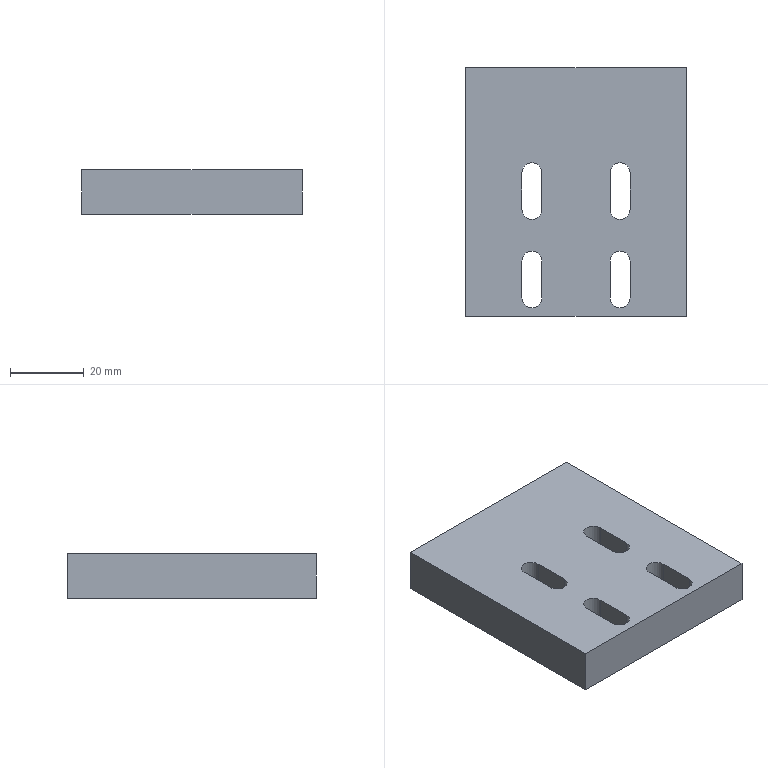Part | SolidWorks | features Cut 1, Extrusion 1, HoleWzd 1 | 1 solid | 30 faces | box 60 x 67.5 x 12 mm | volume 44553 mm3 | plane 14 | cylinder 12 | cone 4 | commonest cylinder face diameters 5.4 x8 4.2 x4
STEP:
#1=CARTESIAN_POINT('',(-15.,21.35,-2.1));
#2=VERTEX_POINT('',#1);
#3=CARTESIAN_POINT('',(-15.,21.35,2.1));
#4=VERTEX_POINT('',#3);
#5=CARTESIAN_POINT('',(-15.,21.35,0.));
#6=DIRECTION('',(0.,1.,0.));
#7=DIRECTION('',(0.,0.,1.));
#8=AXIS2_PLACEMENT_3D('',#5,#6,#7);
#9=CIRCLE('',#8,2.1);
#10=EDGE_CURVE('',#2,#4,#9,.T.);
#11=ORIENTED_EDGE('',*,*,#10,.F.);
#12=CARTESIAN_POINT('',(-15.,33.75,-2.1));
#13=VERTEX_POINT('',#12);
#14=CARTESIAN_POINT('',(-15.,33.75,-2.1));
#15=DIRECTION('',(0.,1.,0.));
#16=VECTOR('',#15,1000.);
#17=LINE('',#14,#16);
#18=EDGE_CURVE('',#2,#13,#17,.T.);
#19=ORIENTED_EDGE('',*,*,#18,.T.);
#20=CARTESIAN_POINT('',(-15.,33.75,2.1));
#21=VERTEX_POINT('',#20);
#22=CARTESIAN_POINT('',(-15.,33.75,0.));
#23=DIRECTION('',(0.,1.,0.));
#24=DIRECTION('',(0.,0.,1.));
#25=AXIS2_PLACEMENT_3D('',#22,#23,#24);
#26=CIRCLE('',#25,2.1);
#27=EDGE_CURVE('',#13,#21,#26,.T.);
#28=ORIENTED_EDGE('',*,*,#27,.T.);
#29=CARTESIAN_POINT('',(-15.,33.75,2.1));
#30=DIRECTION('',(0.,1.,0.));
#31=VECTOR('',#30,1000.);
#32=LINE('',#29,#31);
#33=EDGE_CURVE('',#4,#21,#32,.T.);
#34=ORIENTED_EDGE('',*,*,#33,.F.);
#35=EDGE_LOOP('',(#11,#19,#28,#34));
#36=FACE_OUTER_BOUND('',#35,.T.);
#37=CARTESIAN_POINT('',(-15.,33.75,0.));
#38=DIRECTION('',(0.,1.,0.));
#39=DIRECTION('',(0.,0.,1.));
#40=AXIS2_PLACEMENT_3D('',#37,#38,#39);
#41=CYLINDRICAL_SURFACE('',#40,2.1);
#42=ADVANCED_FACE('',(#36),#41,.F.);
#43=CARTESIAN_POINT('',(-15.,20.088,0.));
#44=VERTEX_POINT('',#43);
#45=CARTESIAN_POINT('',(-15.,21.35,2.1));
#46=DIRECTION('',(0.,0.515,0.8572));
#47=VECTOR('',#46,1000.);
#48=LINE('',#45,#47);
#49=EDGE_CURVE('',#44,#4,#48,.T.);
#50=ORIENTED_EDGE('',*,*,#49,.F.);
#51=CARTESIAN_POINT('',(-15.,21.35,-2.1));
#52=DIRECTION('',(0.,0.515,-0.8572));
#53=VECTOR('',#52,1000.);
#54=LINE('',#51,#53);
#55=EDGE_CURVE('',#44,#2,#54,.T.);
#56=ORIENTED_EDGE('',*,*,#55,.T.);
#57=ORIENTED_EDGE('',*,*,#10,.T.);
#58=EDGE_LOOP('',(#50,#56,#57));
#59=FACE_OUTER_BOUND('',#58,.T.);
#60=CARTESIAN_POINT('',(-15.,21.35,0.));
#61=DIRECTION('',(0.,1.,0.));
#62=DIRECTION('',(0.,0.,1.));
#63=AXIS2_PLACEMENT_3D('',#60,#61,#62);
#64=CONICAL_SURFACE('',#63,2.1,1.03);
#65=ADVANCED_FACE('',(#59),#64,.F.);
#66=CARTESIAN_POINT('',(15.,21.35,-2.1));
#67=VERTEX_POINT('',#66);
#68=CARTESIAN_POINT('',(15.,21.35,2.1));
#69=VERTEX_POINT('',#68);
#70=CARTESIAN_POINT('',(15.,21.35,0.));
#71=DIRECTION('',(0.,1.,0.));
#72=DIRECTION('',(0.,0.,1.));
#73=AXIS2_PLACEMENT_3D('',#70,#71,#72);
#74=CIRCLE('',#73,2.1);
#75=EDGE_CURVE('',#67,#69,#74,.T.);
#76=ORIENTED_EDGE('',*,*,#75,.F.);
#77=CARTESIAN_POINT('',(15.,33.75,-2.1));
#78=VERTEX_POINT('',#77);
#79=CARTESIAN_POINT('',(15.,33.75,-2.1));
#80=DIRECTION('',(0.,1.,0.));
#81=VECTOR('',#80,1000.);
#82=LINE('',#79,#81);
#83=EDGE_CURVE('',#67,#78,#82,.T.);
#84=ORIENTED_EDGE('',*,*,#83,.T.);
#85=CARTESIAN_POINT('',(15.,33.75,2.1));
#86=VERTEX_POINT('',#85);
#87=CARTESIAN_POINT('',(15.,33.75,0.));
#88=DIRECTION('',(0.,1.,0.));
#89=DIRECTION('',(0.,0.,1.));
#90=AXIS2_PLACEMENT_3D('',#87,#88,#89);
#91=CIRCLE('',#90,2.1);
#92=EDGE_CURVE('',#78,#86,#91,.T.);
#93=ORIENTED_EDGE('',*,*,#92,.T.);
#94=CARTESIAN_POINT('',(15.,33.75,2.1));
#95=DIRECTION('',(0.,1.,0.));
#96=VECTOR('',#95,1000.);
#97=LINE('',#94,#96);
#98=EDGE_CURVE('',#69,#86,#97,.T.);
#99=ORIENTED_EDGE('',*,*,#98,.F.);
#100=EDGE_LOOP('',(#76,#84,#93,#99));
#101=FACE_OUTER_BOUND('',#100,.T.);
#102=CARTESIAN_POINT('',(15.,33.75,0.));
#103=DIRECTION('',(0.,1.,0.));
#104=DIRECTION('',(0.,0.,1.));
#105=AXIS2_PLACEMENT_3D('',#102,#103,#104);
#106=CYLINDRICAL_SURFACE('',#105,2.1);
#107=ADVANCED_FACE('',(#101),#106,.F.);
#108=CARTESIAN_POINT('',(15.,20.088,0.));
#109=VERTEX_POINT('',#108);
#110=CARTESIAN_POINT('',(15.,21.35,2.1));
#111=DIRECTION('',(0.,0.515,0.8572));
#112=VECTOR('',#111,1000.);
#113=LINE('',#110,#112);
#114=EDGE_CURVE('',#109,#69,#113,.T.);
#115=ORIENTED_EDGE('',*,*,#114,.F.);
#116=CARTESIAN_POINT('',(15.,21.35,-2.1));
#117=DIRECTION('',(0.,0.515,-0.8572));
#118=VECTOR('',#117,1000.);
#119=LINE('',#116,#118);
#120=EDGE_CURVE('',#109,#67,#119,.T.);
#121=ORIENTED_EDGE('',*,*,#120,.T.);
#122=ORIENTED_EDGE('',*,*,#75,.T.);
#123=EDGE_LOOP('',(#115,#121,#122));
#124=FACE_OUTER_BOUND('',#123,.T.);
#125=CARTESIAN_POINT('',(15.,21.35,0.));
#126=DIRECTION('',(0.,1.,0.));
#127=DIRECTION('',(0.,0.,1.));
#128=AXIS2_PLACEMENT_3D('',#125,#126,#127);
#129=CONICAL_SURFACE('',#128,2.1,1.03);
#130=ADVANCED_FACE('',(#124),#129,.F.);
#131=CARTESIAN_POINT('',(30.,-33.75,-6.));
#132=VERTEX_POINT('',#131);
#133=CARTESIAN_POINT('',(30.,33.75,-6.));
#134=VERTEX_POINT('',#133);
#135=CARTESIAN_POINT('',(30.,33.75,-6.));
#136=DIRECTION('',(0.,1.,0.));
#137=VECTOR('',#136,1000.);
#138=LINE('',#135,#137);
#139=EDGE_CURVE('',#132,#134,#138,.T.);
#140=ORIENTED_EDGE('',*,*,#139,.T.);
#141=CARTESIAN_POINT('',(30.,33.75,6.));
#142=VERTEX_POINT('',#141);
#143=CARTESIAN_POINT('',(30.,33.75,6.));
#144=DIRECTION('',(0.,0.,-1.));
#145=VECTOR('',#144,1000.);
#146=LINE('',#143,#145);
#147=EDGE_CURVE('',#142,#134,#146,.T.);
#148=ORIENTED_EDGE('',*,*,#147,.F.);
#149=CARTESIAN_POINT('',(30.,-33.75,6.));
#150=VERTEX_POINT('',#149);
#151=CARTESIAN_POINT('',(30.,33.75,6.));
#152=DIRECTION('',(0.,1.,0.));
#153=VECTOR('',#152,1000.);
#154=LINE('',#151,#153);
#155=EDGE_CURVE('',#150,#142,#154,.T.);
#156=ORIENTED_EDGE('',*,*,#155,.F.);
#157=CARTESIAN_POINT('',(30.,-33.75,6.));
#158=DIRECTION('',(0.,0.,-1.));
#159=VECTOR('',#158,1000.);
#160=LINE('',#157,#159);
#161=EDGE_CURVE('',#150,#132,#160,.T.);
#162=ORIENTED_EDGE('',*,*,#161,.T.);
#163=EDGE_LOOP('',(#140,#148,#156,#162));
#164=FACE_OUTER_BOUND('',#163,.T.);
#165=CARTESIAN_POINT('',(30.,33.75,6.));
#166=DIRECTION('',(-1.,0.,0.));
#167=DIRECTION('',(0.,-1.,0.));
#168=AXIS2_PLACEMENT_3D('',#165,#166,#167);
#169=PLANE('',#168);
#170=ADVANCED_FACE('',(#164),#169,.F.);
#171=CARTESIAN_POINT('',(-15.,33.75,0.));
#172=DIRECTION('',(0.,1.,0.));
#173=DIRECTION('',(0.,0.,1.));
#174=AXIS2_PLACEMENT_3D('',#171,#172,#173);
#175=CIRCLE('',#174,2.1);
#176=EDGE_CURVE('',#21,#13,#175,.T.);
#177=ORIENTED_EDGE('',*,*,#176,.F.);
#178=ORIENTED_EDGE('',*,*,#27,.F.);
#179=EDGE_LOOP('',(#177,#178));
#180=FACE_BOUND('',#179,.T.);
#181=CARTESIAN_POINT('',(15.,33.75,0.));
#182=DIRECTION('',(0.,1.,0.));
#183=DIRECTION('',(0.,0.,1.));
#184=AXIS2_PLACEMENT_3D('',#181,#182,#183);
#185=CIRCLE('',#184,2.1);
#186=EDGE_CURVE('',#86,#78,#185,.T.);
#187=ORIENTED_EDGE('',*,*,#186,.F.);
#188=ORIENTED_EDGE('',*,*,#92,.F.);
#189=EDGE_LOOP('',(#187,#188));
#190=FACE_BOUND('',#189,.T.);
#191=CARTESIAN_POINT('',(-30.,33.75,-6.));
#192=VERTEX_POINT('',#191);
#193=CARTESIAN_POINT('',(-30.,33.75,-6.));
#194=DIRECTION('',(-1.,0.,0.));
#195=VECTOR('',#194,1000.);
#196=LINE('',#193,#195);
#197=EDGE_CURVE('',#134,#192,#196,.T.);
#198=ORIENTED_EDGE('',*,*,#197,.T.);
#199=CARTESIAN_POINT('',(-30.,33.75,6.));
#200=VERTEX_POINT('',#199);
#201=CARTESIAN_POINT('',(-30.,33.75,6.));
#202=DIRECTION('',(0.,0.,-1.));
#203=VECTOR('',#202,1000.);
#204=LINE('',#201,#203);
#205=EDGE_CURVE('',#200,#192,#204,.T.);
#206=ORIENTED_EDGE('',*,*,#205,.F.);
#207=CARTESIAN_POINT('',(-30.,33.75,6.));
#208=DIRECTION('',(-1.,0.,0.));
#209=VECTOR('',#208,1000.);
#210=LINE('',#207,#209);
#211=EDGE_CURVE('',#142,#200,#210,.T.);
#212=ORIENTED_EDGE('',*,*,#211,.F.);
#213=ORIENTED_EDGE('',*,*,#147,.T.);
#214=EDGE_LOOP('',(#198,#206,#212,#213));
#215=FACE_OUTER_BOUND('',#214,.T.);
#216=CARTESIAN_POINT('',(-30.,33.75,6.));
#217=DIRECTION('',(0.,-1.,0.));
#218=DIRECTION('',(0.,0.,-1.));
#219=AXIS2_PLACEMENT_3D('',#216,#217,#218);
#220=PLANE('',#219);
#221=ADVANCED_FACE('',(#180,#190,#215),#220,.F.);
#222=CARTESIAN_POINT('',(-30.,-33.75,-6.));
#223=VERTEX_POINT('',#222);
#224=CARTESIAN_POINT('',(-30.,33.75,-6.));
#225=DIRECTION('',(0.,-1.,0.));
#226=VECTOR('',#225,1000.);
#227=LINE('',#224,#226);
#228=EDGE_CURVE('',#192,#223,#227,.T.);
#229=ORIENTED_EDGE('',*,*,#228,.T.);
#230=CARTESIAN_POINT('',(-30.,-33.75,6.));
#231=VERTEX_POINT('',#230);
#232=CARTESIAN_POINT('',(-30.,-33.75,6.));
#233=DIRECTION('',(0.,0.,-1.));
#234=VECTOR('',#233,1000.);
#235=LINE('',#232,#234);
#236=EDGE_CURVE('',#231,#223,#235,.T.);
#237=ORIENTED_EDGE('',*,*,#236,.F.);
#238=CARTESIAN_POINT('',(-30.,33.75,6.));
#239=DIRECTION('',(0.,-1.,0.));
#240=VECTOR('',#239,1000.);
#241=LINE('',#238,#240);
#242=EDGE_CURVE('',#200,#231,#241,.T.);
#243=ORIENTED_EDGE('',*,*,#242,.F.);
#244=ORIENTED_EDGE('',*,*,#205,.T.);
#245=EDGE_LOOP('',(#229,#237,#243,#244));
#246=FACE_OUTER_BOUND('',#245,.T.);
#247=CARTESIAN_POINT('',(-30.,33.75,6.));
#248=DIRECTION('',(1.,0.,0.));
#249=DIRECTION('',(0.,1.,0.));
#250=AXIS2_PLACEMENT_3D('',#247,#248,#249);
#251=PLANE('',#250);
#252=ADVANCED_FACE('',(#246),#251,.F.);
#253=CARTESIAN_POINT('',(-30.,-33.75,-6.));
#254=DIRECTION('',(1.,0.,0.));
#255=VECTOR('',#254,1000.);
#256=LINE('',#253,#255);
#257=EDGE_CURVE('',#223,#132,#256,.T.);
#258=ORIENTED_EDGE('',*,*,#257,.T.);
#259=ORIENTED_EDGE('',*,*,#161,.F.);
#260=CARTESIAN_POINT('',(-30.,-33.75,6.));
#261=DIRECTION('',(1.,0.,0.));
#262=VECTOR('',#261,1000.);
#263=LINE('',#260,#262);
#264=EDGE_CURVE('',#231,#150,#263,.T.);
#265=ORIENTED_EDGE('',*,*,#264,.F.);
#266=ORIENTED_EDGE('',*,*,#236,.T.);
#267=EDGE_LOOP('',(#258,#259,#265,#266));
#268=FACE_OUTER_BOUND('',#267,.T.);
#269=CARTESIAN_POINT('',(-30.,-33.75,6.));
#270=DIRECTION('',(0.,1.,0.));
#271=DIRECTION('',(0.,0.,1.));
#272=AXIS2_PLACEMENT_3D('',#269,#270,#271);
#273=PLANE('',#272);
#274=ADVANCED_FACE('',(#268),#273,.F.);
#275=CARTESIAN_POINT('',(14.7,-28.75,6.));
#276=VERTEX_POINT('',#275);
#277=CARTESIAN_POINT('',(9.3,-28.75,6.));
#278=VERTEX_POINT('',#277);
#279=CARTESIAN_POINT('',(12.,-28.75,6.));
#280=DIRECTION('',(0.,0.,-1.));
#281=DIRECTION('',(-1.,0.,0.));
#282=AXIS2_PLACEMENT_3D('',#279,#280,#281);
#283=CIRCLE('',#282,2.7);
#284=EDGE_CURVE('',#276,#278,#283,.T.);
#285=ORIENTED_EDGE('',*,*,#284,.T.);
#286=CARTESIAN_POINT('',(9.3,-18.75,6.));
#287=VERTEX_POINT('',#286);
#288=CARTESIAN_POINT('',(9.3,-28.75,6.));
#289=DIRECTION('',(0.,1.,0.));
#290=VECTOR('',#289,1000.);
#291=LINE('',#288,#290);
#292=EDGE_CURVE('',#278,#287,#291,.T.);
#293=ORIENTED_EDGE('',*,*,#292,.T.);
#294=CARTESIAN_POINT('',(14.7,-18.75,6.));
#295=VERTEX_POINT('',#294);
#296=CARTESIAN_POINT('',(12.,-18.75,6.));
#297=DIRECTION('',(0.,0.,-1.));
#298=DIRECTION('',(-1.,0.,0.));
#299=AXIS2_PLACEMENT_3D('',#296,#297,#298);
#300=CIRCLE('',#299,2.7);
#301=EDGE_CURVE('',#287,#295,#300,.T.);
#302=ORIENTED_EDGE('',*,*,#301,.T.);
#303=CARTESIAN_POINT('',(14.7,-28.75,6.));
#304=DIRECTION('',(0.,-1.,0.));
#305=VECTOR('',#304,1000.);
#306=LINE('',#303,#305);
#307=EDGE_CURVE('',#295,#276,#306,.T.);
#308=ORIENTED_EDGE('',*,*,#307,.T.);
#309=EDGE_LOOP('',(#285,#293,#302,#308));
#310=FACE_BOUND('',#309,.T.);
#311=CARTESIAN_POINT('',(-14.7,5.25,6.));
#312=VERTEX_POINT('',#311);
#313=CARTESIAN_POINT('',(-9.3,5.25,6.));
#314=VERTEX_POINT('',#313);
#315=CARTESIAN_POINT('',(-12.,5.25,6.));
#316=DIRECTION('',(0.,0.,-1.));
#317=DIRECTION('',(-1.,0.,0.));
#318=AXIS2_PLACEMENT_3D('',#315,#316,#317);
#319=CIRCLE('',#318,2.7);
#320=EDGE_CURVE('',#312,#314,#319,.T.);
#321=ORIENTED_EDGE('',*,*,#320,.T.);
#322=CARTESIAN_POINT('',(-9.3,-4.75,6.));
#323=VERTEX_POINT('',#322);
#324=CARTESIAN_POINT('',(-9.3,5.25,6.));
#325=DIRECTION('',(0.,-1.,0.));
#326=VECTOR('',#325,1000.);
#327=LINE('',#324,#326);
#328=EDGE_CURVE('',#314,#323,#327,.T.);
#329=ORIENTED_EDGE('',*,*,#328,.T.);
#330=CARTESIAN_POINT('',(-14.7,-4.75,6.));
#331=VERTEX_POINT('',#330);
#332=CARTESIAN_POINT('',(-12.,-4.75,6.));
#333=DIRECTION('',(0.,0.,-1.));
#334=DIRECTION('',(-1.,0.,0.));
#335=AXIS2_PLACEMENT_3D('',#332,#333,#334);
#336=CIRCLE('',#335,2.7);
#337=EDGE_CURVE('',#323,#331,#336,.T.);
#338=ORIENTED_EDGE('',*,*,#337,.T.);
#339=CARTESIAN_POINT('',(-14.7,5.25,6.));
#340=DIRECTION('',(0.,1.,0.));
#341=VECTOR('',#340,1000.);
#342=LINE('',#339,#341);
#343=EDGE_CURVE('',#331,#312,#342,.T.);
#344=ORIENTED_EDGE('',*,*,#343,.T.);
#345=EDGE_LOOP('',(#321,#329,#338,#344));
#346=FACE_BOUND('',#345,.T.);
#347=CARTESIAN_POINT('',(9.3,5.25,6.));
#348=VERTEX_POINT('',#347);
#349=CARTESIAN_POINT('',(14.7,5.25,6.));
#350=VERTEX_POINT('',#349);
#351=CARTESIAN_POINT('',(12.,5.25,6.));
#352=DIRECTION('',(0.,0.,-1.));
#353=DIRECTION('',(-1.,0.,0.));
#354=AXIS2_PLACEMENT_3D('',#351,#352,#353);
#355=CIRCLE('',#354,2.7);
#356=EDGE_CURVE('',#348,#350,#355,.T.);
#357=ORIENTED_EDGE('',*,*,#356,.T.);
#358=CARTESIAN_POINT('',(14.7,-4.75,6.));
#359=VERTEX_POINT('',#358);
#360=CARTESIAN_POINT('',(14.7,5.25,6.));
#361=DIRECTION('',(0.,-1.,0.));
#362=VECTOR('',#361,1000.);
#363=LINE('',#360,#362);
#364=EDGE_CURVE('',#350,#359,#363,.T.);
#365=ORIENTED_EDGE('',*,*,#364,.T.);
#366=CARTESIAN_POINT('',(9.3,-4.75,6.));
#367=VERTEX_POINT('',#366);
#368=CARTESIAN_POINT('',(12.,-4.75,6.));
#369=DIRECTION('',(0.,0.,-1.));
#370=DIRECTION('',(-1.,0.,0.));
#371=AXIS2_PLACEMENT_3D('',#368,#369,#370);
#372=CIRCLE('',#371,2.7);
#373=EDGE_CURVE('',#359,#367,#372,.T.);
#374=ORIENTED_EDGE('',*,*,#373,.T.);
#375=CARTESIAN_POINT('',(9.3,5.25,6.));
#376=DIRECTION('',(0.,1.,0.));
#377=VECTOR('',#376,1000.);
#378=LINE('',#375,#377);
#379=EDGE_CURVE('',#367,#348,#378,.T.);
#380=ORIENTED_EDGE('',*,*,#379,.T.);
#381=EDGE_LOOP('',(#357,#365,#374,#380));
#382=FACE_BOUND('',#381,.T.);
#383=CARTESIAN_POINT('',(-9.3,-28.75,6.));
#384=VERTEX_POINT('',#383);
#385=CARTESIAN_POINT('',(-14.7,-28.75,6.));
#386=VERTEX_POINT('',#385);
#387=CARTESIAN_POINT('',(-12.,-28.75,6.));
#388=DIRECTION('',(0.,0.,-1.));
#389=DIRECTION('',(-1.,0.,0.));
#390=AXIS2_PLACEMENT_3D('',#387,#388,#389);
#391=CIRCLE('',#390,2.7);
#392=EDGE_CURVE('',#384,#386,#391,.T.);
#393=ORIENTED_EDGE('',*,*,#392,.T.);
#394=CARTESIAN_POINT('',(-14.7,-18.75,6.));
#395=VERTEX_POINT('',#394);
#396=CARTESIAN_POINT('',(-14.7,-28.75,6.));
#397=DIRECTION('',(0.,1.,0.));
#398=VECTOR('',#397,1000.);
#399=LINE('',#396,#398);
#400=EDGE_CURVE('',#386,#395,#399,.T.);
#401=ORIENTED_EDGE('',*,*,#400,.T.);
#402=CARTESIAN_POINT('',(-9.3,-18.75,6.));
#403=VERTEX_POINT('',#402);
#404=CARTESIAN_POINT('',(-12.,-18.75,6.));
#405=DIRECTION('',(0.,0.,-1.));
#406=DIRECTION('',(-1.,0.,0.));
#407=AXIS2_PLACEMENT_3D('',#404,#405,#406);
#408=CIRCLE('',#407,2.7);
#409=EDGE_CURVE('',#395,#403,#408,.T.);
#410=ORIENTED_EDGE('',*,*,#409,.T.);
#411=CARTESIAN_POINT('',(-9.3,-28.75,6.));
#412=DIRECTION('',(0.,-1.,0.));
#413=VECTOR('',#412,1000.);
#414=LINE('',#411,#413);
#415=EDGE_CURVE('',#403,#384,#414,.T.);
#416=ORIENTED_EDGE('',*,*,#415,.T.);
#417=EDGE_LOOP('',(#393,#401,#410,#416));
#418=FACE_BOUND('',#417,.T.);
#419=ORIENTED_EDGE('',*,*,#155,.T.);
#420=ORIENTED_EDGE('',*,*,#211,.T.);
#421=ORIENTED_EDGE('',*,*,#242,.T.);
#422=ORIENTED_EDGE('',*,*,#264,.T.);
#423=EDGE_LOOP('',(#419,#420,#421,#422));
#424=FACE_OUTER_BOUND('',#423,.T.);
#425=CARTESIAN_POINT('',(0.,0.,6.));
#426=DIRECTION('',(0.,0.,1.));
#427=DIRECTION('',(1.,0.,0.));
#428=AXIS2_PLACEMENT_3D('',#425,#426,#427);
#429=PLANE('',#428);
#430=ADVANCED_FACE('',(#310,#346,#382,#418,#424),#429,.T.);
#431=CARTESIAN_POINT('',(9.3,-28.75,-6.));
#432=VERTEX_POINT('',#431);
#433=CARTESIAN_POINT('',(9.3,-18.75,-6.));
#434=VERTEX_POINT('',#433);
#435=CARTESIAN_POINT('',(9.3,-28.75,-6.));
#436=DIRECTION('',(0.,1.,0.));
#437=VECTOR('',#436,1000.);
#438=LINE('',#435,#437);
#439=EDGE_CURVE('',#432,#434,#438,.T.);
#440=ORIENTED_EDGE('',*,*,#439,.F.);
#441=CARTESIAN_POINT('',(14.7,-28.75,-6.));
#442=VERTEX_POINT('',#441);
#443=CARTESIAN_POINT('',(12.,-28.75,-6.));
#444=DIRECTION('',(0.,0.,-1.));
#445=DIRECTION('',(-1.,0.,0.));
#446=AXIS2_PLACEMENT_3D('',#443,#444,#445);
#447=CIRCLE('',#446,2.7);
#448=EDGE_CURVE('',#442,#432,#447,.T.);
#449=ORIENTED_EDGE('',*,*,#448,.F.);
#450=CARTESIAN_POINT('',(14.7,-18.75,-6.));
#451=VERTEX_POINT('',#450);
#452=CARTESIAN_POINT('',(14.7,-28.75,-6.));
#453=DIRECTION('',(0.,-1.,0.));
#454=VECTOR('',#453,1000.);
#455=LINE('',#452,#454);
#456=EDGE_CURVE('',#451,#442,#455,.T.);
#457=ORIENTED_EDGE('',*,*,#456,.F.);
#458=CARTESIAN_POINT('',(12.,-18.75,-6.));
#459=DIRECTION('',(0.,0.,-1.));
#460=DIRECTION('',(-1.,0.,0.));
#461=AXIS2_PLACEMENT_3D('',#458,#459,#460);
#462=CIRCLE('',#461,2.7);
#463=EDGE_CURVE('',#434,#451,#462,.T.);
#464=ORIENTED_EDGE('',*,*,#463,.F.);
#465=EDGE_LOOP('',(#440,#449,#457,#464));
#466=FACE_BOUND('',#465,.T.);
#467=CARTESIAN_POINT('',(-9.3,5.25,-6.));
#468=VERTEX_POINT('',#467);
#469=CARTESIAN_POINT('',(-9.3,-4.75,-6.));
#470=VERTEX_POINT('',#469);
#471=CARTESIAN_POINT('',(-9.3,5.25,-6.));
#472=DIRECTION('',(0.,-1.,0.));
#473=VECTOR('',#472,1000.);
#474=LINE('',#471,#473);
#475=EDGE_CURVE('',#468,#470,#474,.T.);
#476=ORIENTED_EDGE('',*,*,#475,.F.);
#477=CARTESIAN_POINT('',(-14.7,5.25,-6.));
#478=VERTEX_POINT('',#477);
#479=CARTESIAN_POINT('',(-12.,5.25,-6.));
#480=DIRECTION('',(0.,0.,-1.));
#481=DIRECTION('',(-1.,0.,0.));
#482=AXIS2_PLACEMENT_3D('',#479,#480,#481);
#483=CIRCLE('',#482,2.7);
#484=EDGE_CURVE('',#478,#468,#483,.T.);
#485=ORIENTED_EDGE('',*,*,#484,.F.);
#486=CARTESIAN_POINT('',(-14.7,-4.75,-6.));
#487=VERTEX_POINT('',#486);
#488=CARTESIAN_POINT('',(-14.7,5.25,-6.));
#489=DIRECTION('',(0.,1.,0.));
#490=VECTOR('',#489,1000.);
#491=LINE('',#488,#490);
#492=EDGE_CURVE('',#487,#478,#491,.T.);
#493=ORIENTED_EDGE('',*,*,#492,.F.);
#494=CARTESIAN_POINT('',(-12.,-4.75,-6.));
#495=DIRECTION('',(0.,0.,-1.));
#496=DIRECTION('',(-1.,0.,0.));
#497=AXIS2_PLACEMENT_3D('',#494,#495,#496);
#498=CIRCLE('',#497,2.7);
#499=EDGE_CURVE('',#470,#487,#498,.T.);
#500=ORIENTED_EDGE('',*,*,#499,.F.);
#501=EDGE_LOOP('',(#476,#485,#493,#500));
#502=FACE_BOUND('',#501,.T.);
#503=CARTESIAN_POINT('',(14.7,5.25,-6.));
#504=VERTEX_POINT('',#503);
#505=CARTESIAN_POINT('',(14.7,-4.75,-6.));
#506=VERTEX_POINT('',#505);
#507=CARTESIAN_POINT('',(14.7,5.25,-6.));
#508=DIRECTION('',(0.,-1.,0.));
#509=VECTOR('',#508,1000.);
#510=LINE('',#507,#509);
#511=EDGE_CURVE('',#504,#506,#510,.T.);
#512=ORIENTED_EDGE('',*,*,#511,.F.);
#513=CARTESIAN_POINT('',(9.3,5.25,-6.));
#514=VERTEX_POINT('',#513);
#515=CARTESIAN_POINT('',(12.,5.25,-6.));
#516=DIRECTION('',(0.,0.,-1.));
#517=DIRECTION('',(-1.,0.,0.));
#518=AXIS2_PLACEMENT_3D('',#515,#516,#517);
#519=CIRCLE('',#518,2.7);
#520=EDGE_CURVE('',#514,#504,#519,.T.);
#521=ORIENTED_EDGE('',*,*,#520,.F.);
#522=CARTESIAN_POINT('',(9.3,-4.75,-6.));
#523=VERTEX_POINT('',#522);
#524=CARTESIAN_POINT('',(9.3,5.25,-6.));
#525=DIRECTION('',(0.,1.,0.));
#526=VECTOR('',#525,1000.);
#527=LINE('',#524,#526);
#528=EDGE_CURVE('',#523,#514,#527,.T.);
#529=ORIENTED_EDGE('',*,*,#528,.F.);
#530=CARTESIAN_POINT('',(12.,-4.75,-6.));
#531=DIRECTION('',(0.,0.,-1.));
#532=DIRECTION('',(-1.,0.,0.));
#533=AXIS2_PLACEMENT_3D('',#530,#531,#532);
#534=CIRCLE('',#533,2.7);
#535=EDGE_CURVE('',#506,#523,#534,.T.);
#536=ORIENTED_EDGE('',*,*,#535,.F.);
#537=EDGE_LOOP('',(#512,#521,#529,#536));
#538=FACE_BOUND('',#537,.T.);
#539=CARTESIAN_POINT('',(-14.7,-28.75,-6.));
#540=VERTEX_POINT('',#539);
#541=CARTESIAN_POINT('',(-14.7,-18.75,-6.));
#542=VERTEX_POINT('',#541);
#543=CARTESIAN_POINT('',(-14.7,-28.75,-6.));
#544=DIRECTION('',(0.,1.,0.));
#545=VECTOR('',#544,1000.);
#546=LINE('',#543,#545);
#547=EDGE_CURVE('',#540,#542,#546,.T.);
#548=ORIENTED_EDGE('',*,*,#547,.F.);
#549=CARTESIAN_POINT('',(-9.3,-28.75,-6.));
#550=VERTEX_POINT('',#549);
#551=CARTESIAN_POINT('',(-12.,-28.75,-6.));
#552=DIRECTION('',(0.,0.,-1.));
#553=DIRECTION('',(-1.,0.,0.));
#554=AXIS2_PLACEMENT_3D('',#551,#552,#553);
#555=CIRCLE('',#554,2.7);
#556=EDGE_CURVE('',#550,#540,#555,.T.);
#557=ORIENTED_EDGE('',*,*,#556,.F.);
#558=CARTESIAN_POINT('',(-9.3,-18.75,-6.));
#559=VERTEX_POINT('',#558);
#560=CARTESIAN_POINT('',(-9.3,-28.75,-6.));
#561=DIRECTION('',(0.,-1.,0.));
#562=VECTOR('',#561,1000.);
#563=LINE('',#560,#562);
#564=EDGE_CURVE('',#559,#550,#563,.T.);
#565=ORIENTED_EDGE('',*,*,#564,.F.);
#566=CARTESIAN_POINT('',(-12.,-18.75,-6.));
#567=DIRECTION('',(0.,0.,-1.));
#568=DIRECTION('',(-1.,0.,0.));
#569=AXIS2_PLACEMENT_3D('',#566,#567,#568);
#570=CIRCLE('',#569,2.7);
#571=EDGE_CURVE('',#542,#559,#570,.T.);
#572=ORIENTED_EDGE('',*,*,#571,.F.);
#573=EDGE_LOOP('',(#548,#557,#565,#572));
#574=FACE_BOUND('',#573,.T.);
#575=ORIENTED_EDGE('',*,*,#139,.F.);
#576=ORIENTED_EDGE('',*,*,#257,.F.);
#577=ORIENTED_EDGE('',*,*,#228,.F.);
#578=ORIENTED_EDGE('',*,*,#197,.F.);
#579=EDGE_LOOP('',(#575,#576,#577,#578));
#580=FACE_OUTER_BOUND('',#579,.T.);
#581=CARTESIAN_POINT('',(0.,0.,-6.));
#582=DIRECTION('',(0.,0.,1.));
#583=DIRECTION('',(1.,0.,0.));
#584=AXIS2_PLACEMENT_3D('',#581,#582,#583);
#585=PLANE('',#584);
#586=ADVANCED_FACE('',(#466,#502,#538,#574,#580),#585,.F.);
#587=ORIENTED_EDGE('',*,*,#556,.T.);
#588=CARTESIAN_POINT('',(-14.7,-28.75,6.));
#589=DIRECTION('',(0.,0.,-1.));
#590=VECTOR('',#589,1000.);
#591=LINE('',#588,#590);
#592=EDGE_CURVE('',#386,#540,#591,.T.);
#593=ORIENTED_EDGE('',*,*,#592,.F.);
#594=ORIENTED_EDGE('',*,*,#392,.F.);
#595=CARTESIAN_POINT('',(-9.3,-28.75,6.));
#596=DIRECTION('',(0.,0.,-1.));
#597=VECTOR('',#596,1000.);
#598=LINE('',#595,#597);
#599=EDGE_CURVE('',#384,#550,#598,.T.);
#600=ORIENTED_EDGE('',*,*,#599,.T.);
#601=EDGE_LOOP('',(#587,#593,#594,#600));
#602=FACE_OUTER_BOUND('',#601,.T.);
#603=CARTESIAN_POINT('',(-12.,-28.75,6.));
#604=DIRECTION('',(0.,0.,-1.));
#605=DIRECTION('',(-1.,0.,0.));
#606=AXIS2_PLACEMENT_3D('',#603,#604,#605);
#607=CYLINDRICAL_SURFACE('',#606,2.7);
#608=ADVANCED_FACE('',(#602),#607,.F.);
#609=ORIENTED_EDGE('',*,*,#564,.T.);
#610=ORIENTED_EDGE('',*,*,#599,.F.);
#611=ORIENTED_EDGE('',*,*,#415,.F.);
#612=CARTESIAN_POINT('',(-9.3,-18.75,6.));
#613=DIRECTION('',(0.,0.,-1.));
#614=VECTOR('',#613,1000.);
#615=LINE('',#612,#614);
#616=EDGE_CURVE('',#403,#559,#615,.T.);
#617=ORIENTED_EDGE('',*,*,#616,.T.);
#618=EDGE_LOOP('',(#609,#610,#611,#617));
#619=FACE_OUTER_BOUND('',#618,.T.);
#620=CARTESIAN_POINT('',(-9.3,-28.75,6.));
#621=DIRECTION('',(1.,0.,0.));
#622=DIRECTION('',(0.,1.,0.));
#623=AXIS2_PLACEMENT_3D('',#620,#621,#622);
#624=PLANE('',#623);
#625=ADVANCED_FACE('',(#619),#624,.F.);
#626=ORIENTED_EDGE('',*,*,#571,.T.);
#627=ORIENTED_EDGE('',*,*,#616,.F.);
#628=ORIENTED_EDGE('',*,*,#409,.F.);
#629=CARTESIAN_POINT('',(-14.7,-18.75,6.));
#630=DIRECTION('',(0.,0.,-1.));
#631=VECTOR('',#630,1000.);
#632=LINE('',#629,#631);
#633=EDGE_CURVE('',#395,#542,#632,.T.);
#634=ORIENTED_EDGE('',*,*,#633,.T.);
#635=EDGE_LOOP('',(#626,#627,#628,#634));
#636=FACE_OUTER_BOUND('',#635,.T.);
#637=CARTESIAN_POINT('',(-12.,-18.75,6.));
#638=DIRECTION('',(0.,0.,-1.));
#639=DIRECTION('',(-1.,0.,0.));
#640=AXIS2_PLACEMENT_3D('',#637,#638,#639);
#641=CYLINDRICAL_SURFACE('',#640,2.7);
#642=ADVANCED_FACE('',(#636),#641,.F.);
#643=ORIENTED_EDGE('',*,*,#547,.T.);
#644=ORIENTED_EDGE('',*,*,#633,.F.);
#645=ORIENTED_EDGE('',*,*,#400,.F.);
#646=ORIENTED_EDGE('',*,*,#592,.T.);
#647=EDGE_LOOP('',(#643,#644,#645,#646));
#648=FACE_OUTER_BOUND('',#647,.T.);
#649=CARTESIAN_POINT('',(-14.7,-28.75,6.));
#650=DIRECTION('',(-1.,0.,0.));
#651=DIRECTION('',(0.,-1.,0.));
#652=AXIS2_PLACEMENT_3D('',#649,#650,#651);
#653=PLANE('',#652);
#654=ADVANCED_FACE('',(#648),#653,.F.);
#655=ORIENTED_EDGE('',*,*,#520,.T.);
#656=CARTESIAN_POINT('',(14.7,5.25,6.));
#657=DIRECTION('',(0.,0.,-1.));
#658=VECTOR('',#657,1000.);
#659=LINE('',#656,#658);
#660=EDGE_CURVE('',#350,#504,#659,.T.);
#661=ORIENTED_EDGE('',*,*,#660,.F.);
#662=ORIENTED_EDGE('',*,*,#356,.F.);
#663=CARTESIAN_POINT('',(9.3,5.25,6.));
#664=DIRECTION('',(0.,0.,-1.));
#665=VECTOR('',#664,1000.);
#666=LINE('',#663,#665);
#667=EDGE_CURVE('',#348,#514,#666,.T.);
#668=ORIENTED_EDGE('',*,*,#667,.T.);
#669=EDGE_LOOP('',(#655,#661,#662,#668));
#670=FACE_OUTER_BOUND('',#669,.T.);
#671=CARTESIAN_POINT('',(12.,5.25,6.));
#672=DIRECTION('',(0.,0.,-1.));
#673=DIRECTION('',(-1.,0.,0.));
#674=AXIS2_PLACEMENT_3D('',#671,#672,#673);
#675=CYLINDRICAL_SURFACE('',#674,2.7);
#676=ADVANCED_FACE('',(#670),#675,.F.);
#677=ORIENTED_EDGE('',*,*,#528,.T.);
#678=ORIENTED_EDGE('',*,*,#667,.F.);
#679=ORIENTED_EDGE('',*,*,#379,.F.);
#680=CARTESIAN_POINT('',(9.3,-4.75,6.));
#681=DIRECTION('',(0.,0.,-1.));
#682=VECTOR('',#681,1000.);
#683=LINE('',#680,#682);
#684=EDGE_CURVE('',#367,#523,#683,.T.);
#685=ORIENTED_EDGE('',*,*,#684,.T.);
#686=EDGE_LOOP('',(#677,#678,#679,#685));
#687=FACE_OUTER_BOUND('',#686,.T.);
#688=CARTESIAN_POINT('',(9.3,5.25,6.));
#689=DIRECTION('',(-1.,0.,0.));
#690=DIRECTION('',(0.,-1.,0.));
#691=AXIS2_PLACEMENT_3D('',#688,#689,#690);
#692=PLANE('',#691);
#693=ADVANCED_FACE('',(#687),#692,.F.);
#694=ORIENTED_EDGE('',*,*,#535,.T.);
#695=ORIENTED_EDGE('',*,*,#684,.F.);
#696=ORIENTED_EDGE('',*,*,#373,.F.);
#697=CARTESIAN_POINT('',(14.7,-4.75,6.));
#698=DIRECTION('',(0.,0.,-1.));
#699=VECTOR('',#698,1000.);
#700=LINE('',#697,#699);
#701=EDGE_CURVE('',#359,#506,#700,.T.);
#702=ORIENTED_EDGE('',*,*,#701,.T.);
#703=EDGE_LOOP('',(#694,#695,#696,#702));
#704=FACE_OUTER_BOUND('',#703,.T.);
#705=CARTESIAN_POINT('',(12.,-4.75,6.));
#706=DIRECTION('',(0.,0.,-1.));
#707=DIRECTION('',(-1.,0.,0.));
#708=AXIS2_PLACEMENT_3D('',#705,#706,#707);
#709=CYLINDRICAL_SURFACE('',#708,2.7);
#710=ADVANCED_FACE('',(#704),#709,.F.);
#711=ORIENTED_EDGE('',*,*,#511,.T.);
#712=ORIENTED_EDGE('',*,*,#701,.F.);
#713=ORIENTED_EDGE('',*,*,#364,.F.);
#714=ORIENTED_EDGE('',*,*,#660,.T.);
#715=EDGE_LOOP('',(#711,#712,#713,#714));
#716=FACE_OUTER_BOUND('',#715,.T.);
#717=CARTESIAN_POINT('',(14.7,5.25,6.));
#718=DIRECTION('',(1.,0.,0.));
#719=DIRECTION('',(0.,1.,0.));
#720=AXIS2_PLACEMENT_3D('',#717,#718,#719);
#721=PLANE('',#720);
#722=ADVANCED_FACE('',(#716),#721,.F.);
#723=ORIENTED_EDGE('',*,*,#484,.T.);
#724=CARTESIAN_POINT('',(-9.3,5.25,6.));
#725=DIRECTION('',(0.,0.,-1.));
#726=VECTOR('',#725,1000.);
#727=LINE('',#724,#726);
#728=EDGE_CURVE('',#314,#468,#727,.T.);
#729=ORIENTED_EDGE('',*,*,#728,.F.);
#730=ORIENTED_EDGE('',*,*,#320,.F.);
#731=CARTESIAN_POINT('',(-14.7,5.25,6.));
#732=DIRECTION('',(0.,0.,-1.));
#733=VECTOR('',#732,1000.);
#734=LINE('',#731,#733);
#735=EDGE_CURVE('',#312,#478,#734,.T.);
#736=ORIENTED_EDGE('',*,*,#735,.T.);
#737=EDGE_LOOP('',(#723,#729,#730,#736));
#738=FACE_OUTER_BOUND('',#737,.T.);
#739=CARTESIAN_POINT('',(-12.,5.25,6.));
#740=DIRECTION('',(0.,0.,-1.));
#741=DIRECTION('',(-1.,0.,0.));
#742=AXIS2_PLACEMENT_3D('',#739,#740,#741);
#743=CYLINDRICAL_SURFACE('',#742,2.7);
#744=ADVANCED_FACE('',(#738),#743,.F.);
#745=ORIENTED_EDGE('',*,*,#492,.T.);
#746=ORIENTED_EDGE('',*,*,#735,.F.);
#747=ORIENTED_EDGE('',*,*,#343,.F.);
#748=CARTESIAN_POINT('',(-14.7,-4.75,6.));
#749=DIRECTION('',(0.,0.,-1.));
#750=VECTOR('',#749,1000.);
#751=LINE('',#748,#750);
#752=EDGE_CURVE('',#331,#487,#751,.T.);
#753=ORIENTED_EDGE('',*,*,#752,.T.);
#754=EDGE_LOOP('',(#745,#746,#747,#753));
#755=FACE_OUTER_BOUND('',#754,.T.);
#756=CARTESIAN_POINT('',(-14.7,5.25,6.));
#757=DIRECTION('',(-1.,0.,0.));
#758=DIRECTION('',(0.,-1.,0.));
#759=AXIS2_PLACEMENT_3D('',#756,#757,#758);
#760=PLANE('',#759);
#761=ADVANCED_FACE('',(#755),#760,.F.);
#762=ORIENTED_EDGE('',*,*,#499,.T.);
#763=ORIENTED_EDGE('',*,*,#752,.F.);
#764=ORIENTED_EDGE('',*,*,#337,.F.);
#765=CARTESIAN_POINT('',(-9.3,-4.75,6.));
#766=DIRECTION('',(0.,0.,-1.));
#767=VECTOR('',#766,1000.);
#768=LINE('',#765,#767);
#769=EDGE_CURVE('',#323,#470,#768,.T.);
#770=ORIENTED_EDGE('',*,*,#769,.T.);
#771=EDGE_LOOP('',(#762,#763,#764,#770));
#772=FACE_OUTER_BOUND('',#771,.T.);
#773=CARTESIAN_POINT('',(-12.,-4.75,6.));
#774=DIRECTION('',(0.,0.,-1.));
#775=DIRECTION('',(-1.,0.,0.));
#776=AXIS2_PLACEMENT_3D('',#773,#774,#775);
#777=CYLINDRICAL_SURFACE('',#776,2.7);
#778=ADVANCED_FACE('',(#772),#777,.F.);
#779=ORIENTED_EDGE('',*,*,#475,.T.);
#780=ORIENTED_EDGE('',*,*,#769,.F.);
#781=ORIENTED_EDGE('',*,*,#328,.F.);
#782=ORIENTED_EDGE('',*,*,#728,.T.);
#783=EDGE_LOOP('',(#779,#780,#781,#782));
#784=FACE_OUTER_BOUND('',#783,.T.);
#785=CARTESIAN_POINT('',(-9.3,5.25,6.));
#786=DIRECTION('',(1.,0.,0.));
#787=DIRECTION('',(0.,1.,0.));
#788=AXIS2_PLACEMENT_3D('',#785,#786,#787);
#789=PLANE('',#788);
#790=ADVANCED_FACE('',(#784),#789,.F.);
#791=ORIENTED_EDGE('',*,*,#448,.T.);
#792=CARTESIAN_POINT('',(9.3,-28.75,6.));
#793=DIRECTION('',(0.,0.,-1.));
#794=VECTOR('',#793,1000.);
#795=LINE('',#792,#794);
#796=EDGE_CURVE('',#278,#432,#795,.T.);
#797=ORIENTED_EDGE('',*,*,#796,.F.);
#798=ORIENTED_EDGE('',*,*,#284,.F.);
#799=CARTESIAN_POINT('',(14.7,-28.75,6.));
#800=DIRECTION('',(0.,0.,-1.));
#801=VECTOR('',#800,1000.);
#802=LINE('',#799,#801);
#803=EDGE_CURVE('',#276,#442,#802,.T.);
#804=ORIENTED_EDGE('',*,*,#803,.T.);
#805=EDGE_LOOP('',(#791,#797,#798,#804));
#806=FACE_OUTER_BOUND('',#805,.T.);
#807=CARTESIAN_POINT('',(12.,-28.75,6.));
#808=DIRECTION('',(0.,0.,-1.));
#809=DIRECTION('',(-1.,0.,0.));
#810=AXIS2_PLACEMENT_3D('',#807,#808,#809);
#811=CYLINDRICAL_SURFACE('',#810,2.7);
#812=ADVANCED_FACE('',(#806),#811,.F.);
#813=ORIENTED_EDGE('',*,*,#456,.T.);
#814=ORIENTED_EDGE('',*,*,#803,.F.);
#815=ORIENTED_EDGE('',*,*,#307,.F.);
#816=CARTESIAN_POINT('',(14.7,-18.75,6.));
#817=DIRECTION('',(0.,0.,-1.));
#818=VECTOR('',#817,1000.);
#819=LINE('',#816,#818);
#820=EDGE_CURVE('',#295,#451,#819,.T.);
#821=ORIENTED_EDGE('',*,*,#820,.T.);
#822=EDGE_LOOP('',(#813,#814,#815,#821));
#823=FACE_OUTER_BOUND('',#822,.T.);
#824=CARTESIAN_POINT('',(14.7,-28.75,6.));
#825=DIRECTION('',(1.,0.,0.));
#826=DIRECTION('',(0.,1.,0.));
#827=AXIS2_PLACEMENT_3D('',#824,#825,#826);
#828=PLANE('',#827);
#829=ADVANCED_FACE('',(#823),#828,.F.);
#830=ORIENTED_EDGE('',*,*,#463,.T.);
#831=ORIENTED_EDGE('',*,*,#820,.F.);
#832=ORIENTED_EDGE('',*,*,#301,.F.);
#833=CARTESIAN_POINT('',(9.3,-18.75,6.));
#834=DIRECTION('',(0.,0.,-1.));
#835=VECTOR('',#834,1000.);
#836=LINE('',#833,#835);
#837=EDGE_CURVE('',#287,#434,#836,.T.);
#838=ORIENTED_EDGE('',*,*,#837,.T.);
#839=EDGE_LOOP('',(#830,#831,#832,#838));
#840=FACE_OUTER_BOUND('',#839,.T.);
#841=CARTESIAN_POINT('',(12.,-18.75,6.));
#842=DIRECTION('',(0.,0.,-1.));
#843=DIRECTION('',(-1.,0.,0.));
#844=AXIS2_PLACEMENT_3D('',#841,#842,#843);
#845=CYLINDRICAL_SURFACE('',#844,2.7);
#846=ADVANCED_FACE('',(#840),#845,.F.);
#847=ORIENTED_EDGE('',*,*,#439,.T.);
#848=ORIENTED_EDGE('',*,*,#837,.F.);
#849=ORIENTED_EDGE('',*,*,#292,.F.);
#850=ORIENTED_EDGE('',*,*,#796,.T.);
#851=EDGE_LOOP('',(#847,#848,#849,#850));
#852=FACE_OUTER_BOUND('',#851,.T.);
#853=CARTESIAN_POINT('',(9.3,-28.75,6.));
#854=DIRECTION('',(-1.,0.,0.));
#855=DIRECTION('',(0.,-1.,0.));
#856=AXIS2_PLACEMENT_3D('',#853,#854,#855);
#857=PLANE('',#856);
#858=ADVANCED_FACE('',(#852),#857,.F.);
#859=ORIENTED_EDGE('',*,*,#120,.F.);
#860=ORIENTED_EDGE('',*,*,#114,.T.);
#861=CARTESIAN_POINT('',(15.,21.35,0.));
#862=DIRECTION('',(0.,1.,0.));
#863=DIRECTION('',(0.,0.,1.));
#864=AXIS2_PLACEMENT_3D('',#861,#862,#863);
#865=CIRCLE('',#864,2.1);
#866=EDGE_CURVE('',#69,#67,#865,.T.);
#867=ORIENTED_EDGE('',*,*,#866,.T.);
#868=EDGE_LOOP('',(#859,#860,#867));
#869=FACE_OUTER_BOUND('',#868,.T.);
#870=CARTESIAN_POINT('',(15.,21.35,0.));
#871=DIRECTION('',(0.,1.,0.));
#872=DIRECTION('',(0.,0.,1.));
#873=AXIS2_PLACEMENT_3D('',#870,#871,#872);
#874=CONICAL_SURFACE('',#873,2.1,1.03);
#875=ADVANCED_FACE('',(#869),#874,.F.);
#876=ORIENTED_EDGE('',*,*,#83,.F.);
#877=ORIENTED_EDGE('',*,*,#866,.F.);
#878=ORIENTED_EDGE('',*,*,#98,.T.);
#879=ORIENTED_EDGE('',*,*,#186,.T.);
#880=EDGE_LOOP('',(#876,#877,#878,#879));
#881=FACE_OUTER_BOUND('',#880,.T.);
#882=CARTESIAN_POINT('',(15.,33.75,0.));
#883=DIRECTION('',(0.,1.,0.));
#884=DIRECTION('',(0.,0.,1.));
#885=AXIS2_PLACEMENT_3D('',#882,#883,#884);
#886=CYLINDRICAL_SURFACE('',#885,2.1);
#887=ADVANCED_FACE('',(#881),#886,.F.);
#888=ORIENTED_EDGE('',*,*,#55,.F.);
#889=ORIENTED_EDGE('',*,*,#49,.T.);
#890=CARTESIAN_POINT('',(-15.,21.35,0.));
#891=DIRECTION('',(0.,1.,0.));
#892=DIRECTION('',(0.,0.,1.));
#893=AXIS2_PLACEMENT_3D('',#890,#891,#892);
#894=CIRCLE('',#893,2.1);
#895=EDGE_CURVE('',#4,#2,#894,.T.);
#896=ORIENTED_EDGE('',*,*,#895,.T.);
#897=EDGE_LOOP('',(#888,#889,#896));
#898=FACE_OUTER_BOUND('',#897,.T.);
#899=CARTESIAN_POINT('',(-15.,21.35,0.));
#900=DIRECTION('',(0.,1.,0.));
#901=DIRECTION('',(0.,0.,1.));
#902=AXIS2_PLACEMENT_3D('',#899,#900,#901);
#903=CONICAL_SURFACE('',#902,2.1,1.03);
#904=ADVANCED_FACE('',(#898),#903,.F.);
#905=ORIENTED_EDGE('',*,*,#18,.F.);
#906=ORIENTED_EDGE('',*,*,#895,.F.);
#907=ORIENTED_EDGE('',*,*,#33,.T.);
#908=ORIENTED_EDGE('',*,*,#176,.T.);
#909=EDGE_LOOP('',(#905,#906,#907,#908));
#910=FACE_OUTER_BOUND('',#909,.T.);
#911=CARTESIAN_POINT('',(-15.,33.75,0.));
#912=DIRECTION('',(0.,1.,0.));
#913=DIRECTION('',(0.,0.,1.));
#914=AXIS2_PLACEMENT_3D('',#911,#912,#913);
#915=CYLINDRICAL_SURFACE('',#914,2.1);
#916=ADVANCED_FACE('',(#910),#915,.F.);
#917=CLOSED_SHELL('',(#42,#65,#107,#130,#170,#221,#252,#274,#430,#586,#608,#625,#642,#654,#676,#693,#710,#722,#744,#761,#778,#790,#812,#829,#846,#858,#875,#887,#904,#916));
#918=MANIFOLD_SOLID_BREP('',#917);
#919=CARTESIAN_POINT('',(0.,0.,0.));
#920=DIRECTION('',(0.,0.,1.));
#921=DIRECTION('',(1.,0.,0.));
#922=AXIS2_PLACEMENT_3D('',#919,#920,#921);
#923=(LENGTH_UNIT()NAMED_UNIT(*)SI_UNIT(.MILLI.,.METRE.));
#924=UNCERTAINTY_MEASURE_WITH_UNIT(LENGTH_MEASURE(0.00001),#923,'','');
#925=(NAMED_UNIT(*)PLANE_ANGLE_UNIT()SI_UNIT($,.RADIAN.));
#926=(NAMED_UNIT(*)SI_UNIT($,.STERADIAN.)SOLID_ANGLE_UNIT());
#927=(GEOMETRIC_REPRESENTATION_CONTEXT(3)GLOBAL_UNCERTAINTY_ASSIGNED_CONTEXT((#924))GLOBAL_UNIT_ASSIGNED_CONTEXT((#923,#925,#926))REPRESENTATION_CONTEXT('',''));
#928=ADVANCED_BREP_SHAPE_REPRESENTATION('',(#918,#922),#927);